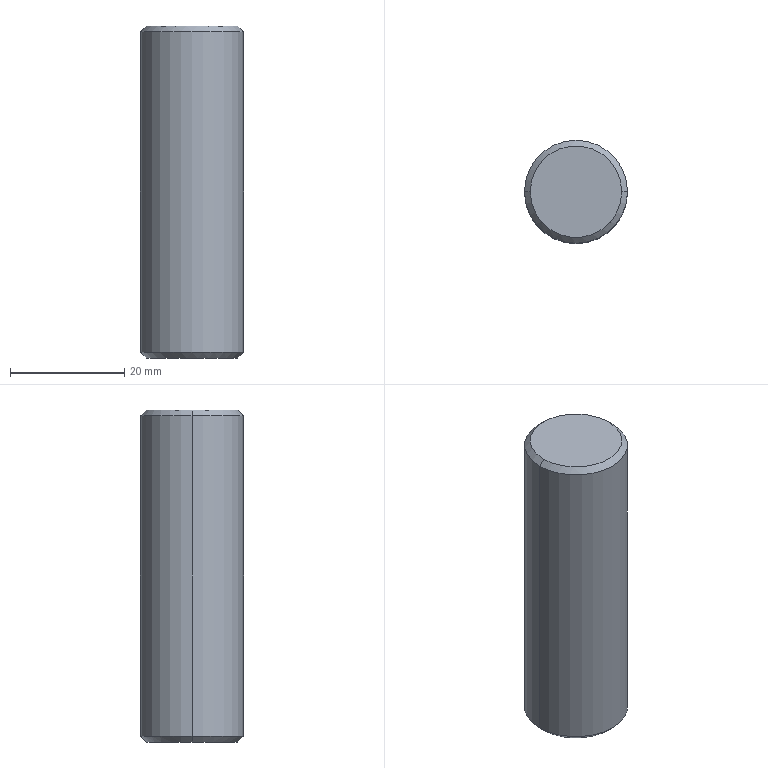Part | STEP file | Ejector guide | 1 solid | 8 faces | box 18 x 18 x 58 mm | volume 14705 mm3 | cone 4 | cylinder 2 | plane 2 | commonest cylinder face diameters 18 x2
STEP:
#1=CARTESIAN_POINT('',(0.,0.,0.));
#2=DIRECTION('',(0.,0.,1.));
#3=DIRECTION('',(1.,0.,0.));
#4=AXIS2_PLACEMENT_3D('',#1,#2,#3);
#5=CARTESIAN_POINT('',(8.,0.,58.));
#6=VERTEX_POINT('',#5);
#7=CARTESIAN_POINT('',(-8.,0.,58.));
#8=VERTEX_POINT('',#7);
#9=CARTESIAN_POINT('',(0.,0.,58.));
#10=DIRECTION('',(0.,0.,1.));
#11=DIRECTION('',(1.,0.,0.));
#12=AXIS2_PLACEMENT_3D('',#9,#10,#11);
#13=CIRCLE('',#12,8.);
#14=CARTESIAN_POINT('',(0.,0.,58.));
#15=DIRECTION('',(0.,0.,-1.));
#16=DIRECTION('',(-1.,0.,0.));
#17=AXIS2_PLACEMENT_3D('',#14,#15,#16);
#18=CONICAL_SURFACE('',#17,8.,0.7854);
#19=CARTESIAN_POINT('',(3.142,0.));
#20=DIRECTION('',(-1.,0.));
#21=VECTOR('',#20,1.);
#22=LINE('',#19,#21);
#23=(GEOMETRIC_REPRESENTATION_CONTEXT(2)PARAMETRIC_REPRESENTATION_CONTEXT()REPRESENTATION_CONTEXT('',''));
#24=DEFINITIONAL_REPRESENTATION('',(#22),#23);
#25=PCURVE('',#18,#24);
#26=CARTESIAN_POINT('',(0.,0.,58.));
#27=DIRECTION('',(0.,0.,1.));
#28=DIRECTION('',(1.,0.,0.));
#29=AXIS2_PLACEMENT_3D('',#26,#27,#28);
#30=PLANE('',#29);
#31=CARTESIAN_POINT('',(0.,0.));
#32=DIRECTION('',(1.,0.));
#33=AXIS2_PLACEMENT_2D('',#31,#32);
#34=CIRCLE('',#33,8.);
#35=(GEOMETRIC_REPRESENTATION_CONTEXT(2)PARAMETRIC_REPRESENTATION_CONTEXT()REPRESENTATION_CONTEXT('',''));
#36=DEFINITIONAL_REPRESENTATION('',(#34),#35);
#37=PCURVE('',#30,#36);
#38=SURFACE_CURVE('',#13,(#25,#37),.PCURVE_S1.);
#39=EDGE_CURVE('',#6,#8,#38,.T.);
#40=ORIENTED_EDGE('',*,*,#39,.F.);
#41=CARTESIAN_POINT('',(9.,0.,57.));
#42=VERTEX_POINT('',#41);
#43=CARTESIAN_POINT('',(8.,0.,58.));
#44=DIRECTION('',(0.7071,0.,-0.7071));
#45=VECTOR('',#44,1.);
#46=LINE('',#43,#45);
#47=CARTESIAN_POINT('',(3.142,0.));
#48=DIRECTION('',(0.,1.));
#49=VECTOR('',#48,1.);
#50=LINE('',#47,#49);
#51=(GEOMETRIC_REPRESENTATION_CONTEXT(2)PARAMETRIC_REPRESENTATION_CONTEXT()REPRESENTATION_CONTEXT('',''));
#52=DEFINITIONAL_REPRESENTATION('',(#50),#51);
#53=PCURVE('',#18,#52);
#54=CARTESIAN_POINT('',(0.,0.,58.));
#55=DIRECTION('',(0.,0.,-1.));
#56=DIRECTION('',(-1.,0.,0.));
#57=AXIS2_PLACEMENT_3D('',#54,#55,#56);
#58=CONICAL_SURFACE('',#57,8.,0.7854);
#59=CARTESIAN_POINT('',(3.142,0.));
#60=DIRECTION('',(0.,1.));
#61=VECTOR('',#60,1.);
#62=LINE('',#59,#61);
#63=(GEOMETRIC_REPRESENTATION_CONTEXT(2)PARAMETRIC_REPRESENTATION_CONTEXT()REPRESENTATION_CONTEXT('',''));
#64=DEFINITIONAL_REPRESENTATION('',(#62),#63);
#65=PCURVE('',#58,#64);
#66=SURFACE_CURVE('',#46,(#53,#65),.PCURVE_S1.);
#67=EDGE_CURVE('',#6,#42,#66,.T.);
#68=ORIENTED_EDGE('',*,*,#67,.T.);
#69=CARTESIAN_POINT('',(-9.,0.,57.));
#70=VERTEX_POINT('',#69);
#71=CARTESIAN_POINT('',(0.,0.,57.));
#72=DIRECTION('',(0.,0.,-1.));
#73=DIRECTION('',(1.,0.,0.));
#74=AXIS2_PLACEMENT_3D('',#71,#72,#73);
#75=CIRCLE('',#74,9.);
#76=CARTESIAN_POINT('',(-3.142,1.));
#77=DIRECTION('',(1.,0.));
#78=VECTOR('',#77,1.);
#79=LINE('',#76,#78);
#80=(GEOMETRIC_REPRESENTATION_CONTEXT(2)PARAMETRIC_REPRESENTATION_CONTEXT()REPRESENTATION_CONTEXT('',''));
#81=DEFINITIONAL_REPRESENTATION('',(#79),#80);
#82=PCURVE('',#18,#81);
#83=CARTESIAN_POINT('',(0.,0.,58.));
#84=DIRECTION('',(0.,0.,-1.));
#85=DIRECTION('',(-1.,0.,0.));
#86=AXIS2_PLACEMENT_3D('',#83,#84,#85);
#87=CYLINDRICAL_SURFACE('',#86,9.);
#88=CARTESIAN_POINT('',(-3.142,1.));
#89=DIRECTION('',(1.,0.));
#90=VECTOR('',#89,1.);
#91=LINE('',#88,#90);
#92=(GEOMETRIC_REPRESENTATION_CONTEXT(2)PARAMETRIC_REPRESENTATION_CONTEXT()REPRESENTATION_CONTEXT('',''));
#93=DEFINITIONAL_REPRESENTATION('',(#91),#92);
#94=PCURVE('',#87,#93);
#95=SURFACE_CURVE('',#75,(#82,#94),.PCURVE_S1.);
#96=EDGE_CURVE('',#70,#42,#95,.T.);
#97=ORIENTED_EDGE('',*,*,#96,.F.);
#98=CARTESIAN_POINT('',(-8.,0.,58.));
#99=DIRECTION('',(-0.7071,0.,-0.7071));
#100=VECTOR('',#99,1.);
#101=LINE('',#98,#100);
#102=CARTESIAN_POINT('',(0.,0.));
#103=DIRECTION('',(0.,1.));
#104=VECTOR('',#103,1.);
#105=LINE('',#102,#104);
#106=(GEOMETRIC_REPRESENTATION_CONTEXT(2)PARAMETRIC_REPRESENTATION_CONTEXT()REPRESENTATION_CONTEXT('',''));
#107=DEFINITIONAL_REPRESENTATION('',(#105),#106);
#108=PCURVE('',#18,#107);
#109=CARTESIAN_POINT('',(6.283,0.));
#110=DIRECTION('',(0.,1.));
#111=VECTOR('',#110,1.);
#112=LINE('',#109,#111);
#113=(GEOMETRIC_REPRESENTATION_CONTEXT(2)PARAMETRIC_REPRESENTATION_CONTEXT()REPRESENTATION_CONTEXT('',''));
#114=DEFINITIONAL_REPRESENTATION('',(#112),#113);
#115=PCURVE('',#58,#114);
#116=SURFACE_CURVE('',#101,(#108,#115),.PCURVE_S1.);
#117=EDGE_CURVE('',#8,#70,#116,.T.);
#118=ORIENTED_EDGE('',*,*,#117,.F.);
#119=EDGE_LOOP('',(#40,#68,#97,#118));
#120=FACE_BOUND('',#119,.T.);
#121=ADVANCED_FACE('',(#120),#18,.T.);
#122=CARTESIAN_POINT('',(-8.,0.,0.));
#123=VERTEX_POINT('',#122);
#124=CARTESIAN_POINT('',(8.,0.,0.));
#125=VERTEX_POINT('',#124);
#126=CARTESIAN_POINT('',(0.,0.,0.));
#127=DIRECTION('',(0.,0.,-1.));
#128=DIRECTION('',(1.,0.,0.));
#129=AXIS2_PLACEMENT_3D('',#126,#127,#128);
#130=CIRCLE('',#129,8.);
#131=CARTESIAN_POINT('',(0.,0.,1.));
#132=DIRECTION('',(0.,0.,1.));
#133=DIRECTION('',(1.,0.,0.));
#134=AXIS2_PLACEMENT_3D('',#131,#132,#133);
#135=CONICAL_SURFACE('',#134,9.,0.7854);
#136=CARTESIAN_POINT('',(6.283,-1.));
#137=DIRECTION('',(-1.,0.));
#138=VECTOR('',#137,1.);
#139=LINE('',#136,#138);
#140=(GEOMETRIC_REPRESENTATION_CONTEXT(2)PARAMETRIC_REPRESENTATION_CONTEXT()REPRESENTATION_CONTEXT('',''));
#141=DEFINITIONAL_REPRESENTATION('',(#139),#140);
#142=PCURVE('',#135,#141);
#143=CARTESIAN_POINT('',(0.,0.,0.));
#144=DIRECTION('',(0.,0.,1.));
#145=DIRECTION('',(1.,0.,0.));
#146=AXIS2_PLACEMENT_3D('',#143,#144,#145);
#147=PLANE('',#146);
#148=CARTESIAN_POINT('',(8.,0.));
#149=CARTESIAN_POINT('',(8.,-13.856));
#150=CARTESIAN_POINT('',(-4.,-6.928));
#151=CARTESIAN_POINT('',(-16.,0.));
#152=CARTESIAN_POINT('',(-4.,6.928));
#153=CARTESIAN_POINT('',(8.,13.856));
#154=CARTESIAN_POINT('',(8.,0.));
#155=(BOUNDED_CURVE()B_SPLINE_CURVE(2,(#148,#149,#150,#151,#152,#153,#154),.UNSPECIFIED.,.T.,.F.)B_SPLINE_CURVE_WITH_KNOTS((1,2,2,2,2,1),(-2.094,0.,2.094,4.189,6.283,8.378),.UNSPECIFIED.)CURVE()GEOMETRIC_REPRESENTATION_ITEM()RATIONAL_B_SPLINE_CURVE((1.,0.5,1.,0.5,1.,0.5,1.))REPRESENTATION_ITEM(''));
#156=(GEOMETRIC_REPRESENTATION_CONTEXT(2)PARAMETRIC_REPRESENTATION_CONTEXT()REPRESENTATION_CONTEXT('',''));
#157=DEFINITIONAL_REPRESENTATION('',(#155),#156);
#158=PCURVE('',#147,#157);
#159=SURFACE_CURVE('',#130,(#142,#158),.PCURVE_S1.);
#160=EDGE_CURVE('',#123,#125,#159,.T.);
#161=ORIENTED_EDGE('',*,*,#160,.F.);
#162=CARTESIAN_POINT('',(-9.,0.,1.));
#163=VERTEX_POINT('',#162);
#164=CARTESIAN_POINT('',(-9.,0.,1.));
#165=DIRECTION('',(-0.7071,0.,0.7071));
#166=VECTOR('',#165,1.);
#167=LINE('',#164,#166);
#168=CARTESIAN_POINT('',(3.142,0.));
#169=DIRECTION('',(0.,1.));
#170=VECTOR('',#169,1.);
#171=LINE('',#168,#170);
#172=(GEOMETRIC_REPRESENTATION_CONTEXT(2)PARAMETRIC_REPRESENTATION_CONTEXT()REPRESENTATION_CONTEXT('',''));
#173=DEFINITIONAL_REPRESENTATION('',(#171),#172);
#174=PCURVE('',#135,#173);
#175=CARTESIAN_POINT('',(0.,0.,1.));
#176=DIRECTION('',(0.,0.,1.));
#177=DIRECTION('',(1.,0.,0.));
#178=AXIS2_PLACEMENT_3D('',#175,#176,#177);
#179=CONICAL_SURFACE('',#178,9.,0.7854);
#180=CARTESIAN_POINT('',(3.142,0.));
#181=DIRECTION('',(0.,1.));
#182=VECTOR('',#181,1.);
#183=LINE('',#180,#182);
#184=(GEOMETRIC_REPRESENTATION_CONTEXT(2)PARAMETRIC_REPRESENTATION_CONTEXT()REPRESENTATION_CONTEXT('',''));
#185=DEFINITIONAL_REPRESENTATION('',(#183),#184);
#186=PCURVE('',#179,#185);
#187=SURFACE_CURVE('',#167,(#174,#186),.PCURVE_S1.);
#188=EDGE_CURVE('',#123,#163,#187,.T.);
#189=ORIENTED_EDGE('',*,*,#188,.T.);
#190=CARTESIAN_POINT('',(9.,0.,1.));
#191=VERTEX_POINT('',#190);
#192=CARTESIAN_POINT('',(0.,0.,1.));
#193=DIRECTION('',(0.,0.,1.));
#194=DIRECTION('',(1.,0.,0.));
#195=AXIS2_PLACEMENT_3D('',#192,#193,#194);
#196=CIRCLE('',#195,9.);
#197=CARTESIAN_POINT('',(0.,0.));
#198=DIRECTION('',(1.,0.));
#199=VECTOR('',#198,1.);
#200=LINE('',#197,#199);
#201=(GEOMETRIC_REPRESENTATION_CONTEXT(2)PARAMETRIC_REPRESENTATION_CONTEXT()REPRESENTATION_CONTEXT('',''));
#202=DEFINITIONAL_REPRESENTATION('',(#200),#201);
#203=PCURVE('',#135,#202);
#204=CARTESIAN_POINT('',(3.142,57.));
#205=DIRECTION('',(-1.,0.));
#206=VECTOR('',#205,1.);
#207=LINE('',#204,#206);
#208=(GEOMETRIC_REPRESENTATION_CONTEXT(2)PARAMETRIC_REPRESENTATION_CONTEXT()REPRESENTATION_CONTEXT('',''));
#209=DEFINITIONAL_REPRESENTATION('',(#207),#208);
#210=PCURVE('',#87,#209);
#211=SURFACE_CURVE('',#196,(#203,#210),.PCURVE_S1.);
#212=EDGE_CURVE('',#191,#163,#211,.T.);
#213=ORIENTED_EDGE('',*,*,#212,.F.);
#214=CARTESIAN_POINT('',(9.,0.,1.));
#215=DIRECTION('',(0.7071,0.,0.7071));
#216=VECTOR('',#215,1.);
#217=LINE('',#214,#216);
#218=CARTESIAN_POINT('',(0.,0.));
#219=DIRECTION('',(0.,1.));
#220=VECTOR('',#219,1.);
#221=LINE('',#218,#220);
#222=(GEOMETRIC_REPRESENTATION_CONTEXT(2)PARAMETRIC_REPRESENTATION_CONTEXT()REPRESENTATION_CONTEXT('',''));
#223=DEFINITIONAL_REPRESENTATION('',(#221),#222);
#224=PCURVE('',#135,#223);
#225=CARTESIAN_POINT('',(6.283,0.));
#226=DIRECTION('',(0.,1.));
#227=VECTOR('',#226,1.);
#228=LINE('',#225,#227);
#229=(GEOMETRIC_REPRESENTATION_CONTEXT(2)PARAMETRIC_REPRESENTATION_CONTEXT()REPRESENTATION_CONTEXT('',''));
#230=DEFINITIONAL_REPRESENTATION('',(#228),#229);
#231=PCURVE('',#179,#230);
#232=SURFACE_CURVE('',#217,(#224,#231),.PCURVE_S1.);
#233=EDGE_CURVE('',#125,#191,#232,.T.);
#234=ORIENTED_EDGE('',*,*,#233,.F.);
#235=EDGE_LOOP('',(#161,#189,#213,#234));
#236=FACE_BOUND('',#235,.T.);
#237=ADVANCED_FACE('',(#236),#135,.T.);
#238=ORIENTED_EDGE('',*,*,#96,.T.);
#239=CARTESIAN_POINT('',(9.,0.,58.));
#240=DIRECTION('',(0.,0.,-1.));
#241=VECTOR('',#240,1.);
#242=LINE('',#239,#241);
#243=CARTESIAN_POINT('',(3.142,0.));
#244=DIRECTION('',(0.,1.));
#245=VECTOR('',#244,1.);
#246=LINE('',#243,#245);
#247=(GEOMETRIC_REPRESENTATION_CONTEXT(2)PARAMETRIC_REPRESENTATION_CONTEXT()REPRESENTATION_CONTEXT('',''));
#248=DEFINITIONAL_REPRESENTATION('',(#246),#247);
#249=PCURVE('',#87,#248);
#250=CARTESIAN_POINT('',(0.,0.,58.));
#251=DIRECTION('',(0.,0.,-1.));
#252=DIRECTION('',(-1.,0.,0.));
#253=AXIS2_PLACEMENT_3D('',#250,#251,#252);
#254=CYLINDRICAL_SURFACE('',#253,9.);
#255=CARTESIAN_POINT('',(3.142,0.));
#256=DIRECTION('',(0.,1.));
#257=VECTOR('',#256,1.);
#258=LINE('',#255,#257);
#259=(GEOMETRIC_REPRESENTATION_CONTEXT(2)PARAMETRIC_REPRESENTATION_CONTEXT()REPRESENTATION_CONTEXT('',''));
#260=DEFINITIONAL_REPRESENTATION('',(#258),#259);
#261=PCURVE('',#254,#260);
#262=SURFACE_CURVE('',#242,(#249,#261),.PCURVE_S1.);
#263=EDGE_CURVE('',#42,#191,#262,.T.);
#264=ORIENTED_EDGE('',*,*,#263,.T.);
#265=ORIENTED_EDGE('',*,*,#212,.T.);
#266=CARTESIAN_POINT('',(-9.,0.,58.));
#267=DIRECTION('',(0.,0.,-1.));
#268=VECTOR('',#267,1.);
#269=LINE('',#266,#268);
#270=CARTESIAN_POINT('',(0.,0.));
#271=DIRECTION('',(0.,1.));
#272=VECTOR('',#271,1.);
#273=LINE('',#270,#272);
#274=(GEOMETRIC_REPRESENTATION_CONTEXT(2)PARAMETRIC_REPRESENTATION_CONTEXT()REPRESENTATION_CONTEXT('',''));
#275=DEFINITIONAL_REPRESENTATION('',(#273),#274);
#276=PCURVE('',#87,#275);
#277=CARTESIAN_POINT('',(6.283,0.));
#278=DIRECTION('',(0.,1.));
#279=VECTOR('',#278,1.);
#280=LINE('',#277,#279);
#281=(GEOMETRIC_REPRESENTATION_CONTEXT(2)PARAMETRIC_REPRESENTATION_CONTEXT()REPRESENTATION_CONTEXT('',''));
#282=DEFINITIONAL_REPRESENTATION('',(#280),#281);
#283=PCURVE('',#254,#282);
#284=SURFACE_CURVE('',#269,(#276,#283),.PCURVE_S1.);
#285=EDGE_CURVE('',#70,#163,#284,.T.);
#286=ORIENTED_EDGE('',*,*,#285,.F.);
#287=EDGE_LOOP('',(#238,#264,#265,#286));
#288=FACE_BOUND('',#287,.T.);
#289=ADVANCED_FACE('',(#288),#87,.T.);
#290=ORIENTED_EDGE('',*,*,#263,.F.);
#291=CARTESIAN_POINT('',(0.,0.,57.));
#292=DIRECTION('',(0.,0.,-1.));
#293=DIRECTION('',(1.,0.,0.));
#294=AXIS2_PLACEMENT_3D('',#291,#292,#293);
#295=CIRCLE('',#294,9.);
#296=CARTESIAN_POINT('',(3.142,1.));
#297=DIRECTION('',(1.,0.));
#298=VECTOR('',#297,1.);
#299=LINE('',#296,#298);
#300=(GEOMETRIC_REPRESENTATION_CONTEXT(2)PARAMETRIC_REPRESENTATION_CONTEXT()REPRESENTATION_CONTEXT('',''));
#301=DEFINITIONAL_REPRESENTATION('',(#299),#300);
#302=PCURVE('',#254,#301);
#303=CARTESIAN_POINT('',(3.142,1.));
#304=DIRECTION('',(1.,0.));
#305=VECTOR('',#304,1.);
#306=LINE('',#303,#305);
#307=(GEOMETRIC_REPRESENTATION_CONTEXT(2)PARAMETRIC_REPRESENTATION_CONTEXT()REPRESENTATION_CONTEXT('',''));
#308=DEFINITIONAL_REPRESENTATION('',(#306),#307);
#309=PCURVE('',#58,#308);
#310=SURFACE_CURVE('',#295,(#302,#309),.PCURVE_S1.);
#311=EDGE_CURVE('',#42,#70,#310,.T.);
#312=ORIENTED_EDGE('',*,*,#311,.T.);
#313=ORIENTED_EDGE('',*,*,#285,.T.);
#314=CARTESIAN_POINT('',(0.,0.,1.));
#315=DIRECTION('',(0.,0.,1.));
#316=DIRECTION('',(1.,0.,0.));
#317=AXIS2_PLACEMENT_3D('',#314,#315,#316);
#318=CIRCLE('',#317,9.);
#319=CARTESIAN_POINT('',(9.425,57.));
#320=DIRECTION('',(-1.,0.));
#321=VECTOR('',#320,1.);
#322=LINE('',#319,#321);
#323=(GEOMETRIC_REPRESENTATION_CONTEXT(2)PARAMETRIC_REPRESENTATION_CONTEXT()REPRESENTATION_CONTEXT('',''));
#324=DEFINITIONAL_REPRESENTATION('',(#322),#323);
#325=PCURVE('',#254,#324);
#326=CARTESIAN_POINT('',(0.,0.));
#327=DIRECTION('',(1.,0.));
#328=VECTOR('',#327,1.);
#329=LINE('',#326,#328);
#330=(GEOMETRIC_REPRESENTATION_CONTEXT(2)PARAMETRIC_REPRESENTATION_CONTEXT()REPRESENTATION_CONTEXT('',''));
#331=DEFINITIONAL_REPRESENTATION('',(#329),#330);
#332=PCURVE('',#179,#331);
#333=SURFACE_CURVE('',#318,(#325,#332),.PCURVE_S1.);
#334=EDGE_CURVE('',#163,#191,#333,.T.);
#335=ORIENTED_EDGE('',*,*,#334,.T.);
#336=EDGE_LOOP('',(#290,#312,#313,#335));
#337=FACE_BOUND('',#336,.T.);
#338=ADVANCED_FACE('',(#337),#254,.T.);
#339=CARTESIAN_POINT('',(0.,0.,58.));
#340=DIRECTION('',(0.,0.,1.));
#341=DIRECTION('',(1.,0.,0.));
#342=AXIS2_PLACEMENT_3D('',#339,#340,#341);
#343=CIRCLE('',#342,8.);
#344=CARTESIAN_POINT('',(0.,0.));
#345=DIRECTION('',(1.,0.));
#346=AXIS2_PLACEMENT_2D('',#344,#345);
#347=CIRCLE('',#346,8.);
#348=(GEOMETRIC_REPRESENTATION_CONTEXT(2)PARAMETRIC_REPRESENTATION_CONTEXT()REPRESENTATION_CONTEXT('',''));
#349=DEFINITIONAL_REPRESENTATION('',(#347),#348);
#350=PCURVE('',#30,#349);
#351=CARTESIAN_POINT('',(9.425,0.));
#352=DIRECTION('',(-1.,0.));
#353=VECTOR('',#352,1.);
#354=LINE('',#351,#353);
#355=(GEOMETRIC_REPRESENTATION_CONTEXT(2)PARAMETRIC_REPRESENTATION_CONTEXT()REPRESENTATION_CONTEXT('',''));
#356=DEFINITIONAL_REPRESENTATION('',(#354),#355);
#357=PCURVE('',#58,#356);
#358=SURFACE_CURVE('',#343,(#350,#357),.PCURVE_S1.);
#359=EDGE_CURVE('',#8,#6,#358,.T.);
#360=ORIENTED_EDGE('',*,*,#359,.T.);
#361=ORIENTED_EDGE('',*,*,#39,.T.);
#362=EDGE_LOOP('',(#360,#361));
#363=FACE_BOUND('',#362,.T.);
#364=ADVANCED_FACE('',(#363),#30,.T.);
#365=CARTESIAN_POINT('',(0.,0.,0.));
#366=DIRECTION('',(0.,0.,-1.));
#367=DIRECTION('',(1.,0.,0.));
#368=AXIS2_PLACEMENT_3D('',#365,#366,#367);
#369=CIRCLE('',#368,8.);
#370=CARTESIAN_POINT('',(8.,0.));
#371=CARTESIAN_POINT('',(8.,-13.856));
#372=CARTESIAN_POINT('',(-4.,-6.928));
#373=CARTESIAN_POINT('',(-16.,0.));
#374=CARTESIAN_POINT('',(-4.,6.928));
#375=CARTESIAN_POINT('',(8.,13.856));
#376=CARTESIAN_POINT('',(8.,0.));
#377=(BOUNDED_CURVE()B_SPLINE_CURVE(2,(#370,#371,#372,#373,#374,#375,#376),.UNSPECIFIED.,.T.,.F.)B_SPLINE_CURVE_WITH_KNOTS((1,2,2,2,2,1),(-2.094,0.,2.094,4.189,6.283,8.378),.UNSPECIFIED.)CURVE()GEOMETRIC_REPRESENTATION_ITEM()RATIONAL_B_SPLINE_CURVE((1.,0.5,1.,0.5,1.,0.5,1.))REPRESENTATION_ITEM(''));
#378=(GEOMETRIC_REPRESENTATION_CONTEXT(2)PARAMETRIC_REPRESENTATION_CONTEXT()REPRESENTATION_CONTEXT('',''));
#379=DEFINITIONAL_REPRESENTATION('',(#377),#378);
#380=PCURVE('',#147,#379);
#381=CARTESIAN_POINT('',(6.283,-1.));
#382=DIRECTION('',(-1.,0.));
#383=VECTOR('',#382,1.);
#384=LINE('',#381,#383);
#385=(GEOMETRIC_REPRESENTATION_CONTEXT(2)PARAMETRIC_REPRESENTATION_CONTEXT()REPRESENTATION_CONTEXT('',''));
#386=DEFINITIONAL_REPRESENTATION('',(#384),#385);
#387=PCURVE('',#179,#386);
#388=SURFACE_CURVE('',#369,(#380,#387),.PCURVE_S1.);
#389=EDGE_CURVE('',#125,#123,#388,.T.);
#390=ORIENTED_EDGE('',*,*,#389,.T.);
#391=ORIENTED_EDGE('',*,*,#160,.T.);
#392=EDGE_LOOP('',(#390,#391));
#393=FACE_BOUND('',#392,.T.);
#394=ADVANCED_FACE('',(#393),#147,.F.);
#395=ORIENTED_EDGE('',*,*,#188,.F.);
#396=ORIENTED_EDGE('',*,*,#389,.F.);
#397=ORIENTED_EDGE('',*,*,#233,.T.);
#398=ORIENTED_EDGE('',*,*,#334,.F.);
#399=EDGE_LOOP('',(#395,#396,#397,#398));
#400=FACE_BOUND('',#399,.T.);
#401=ADVANCED_FACE('',(#400),#179,.T.);
#402=ORIENTED_EDGE('',*,*,#67,.F.);
#403=ORIENTED_EDGE('',*,*,#359,.F.);
#404=ORIENTED_EDGE('',*,*,#117,.T.);
#405=ORIENTED_EDGE('',*,*,#311,.F.);
#406=EDGE_LOOP('',(#402,#403,#404,#405));
#407=FACE_BOUND('',#406,.T.);
#408=ADVANCED_FACE('',(#407),#58,.T.);
#409=CLOSED_SHELL('',(#121,#237,#289,#338,#364,#394,#401,#408));
#410=MANIFOLD_SOLID_BREP('',#409);
#411=(LENGTH_UNIT()NAMED_UNIT(*)SI_UNIT(.MILLI.,.METRE.));
#412=UNCERTAINTY_MEASURE_WITH_UNIT(LENGTH_MEASURE(0.0000001),#411,'','');
#413=(NAMED_UNIT(*)PLANE_ANGLE_UNIT()SI_UNIT($,.RADIAN.));
#414=(NAMED_UNIT(*)SI_UNIT($,.STERADIAN.)SOLID_ANGLE_UNIT());
#415=(GEOMETRIC_REPRESENTATION_CONTEXT(3)GLOBAL_UNCERTAINTY_ASSIGNED_CONTEXT((#412))GLOBAL_UNIT_ASSIGNED_CONTEXT((#411,#413,#414))REPRESENTATION_CONTEXT('',''));
#416=ADVANCED_BREP_SHAPE_REPRESENTATION('',(#4,#410),#415);